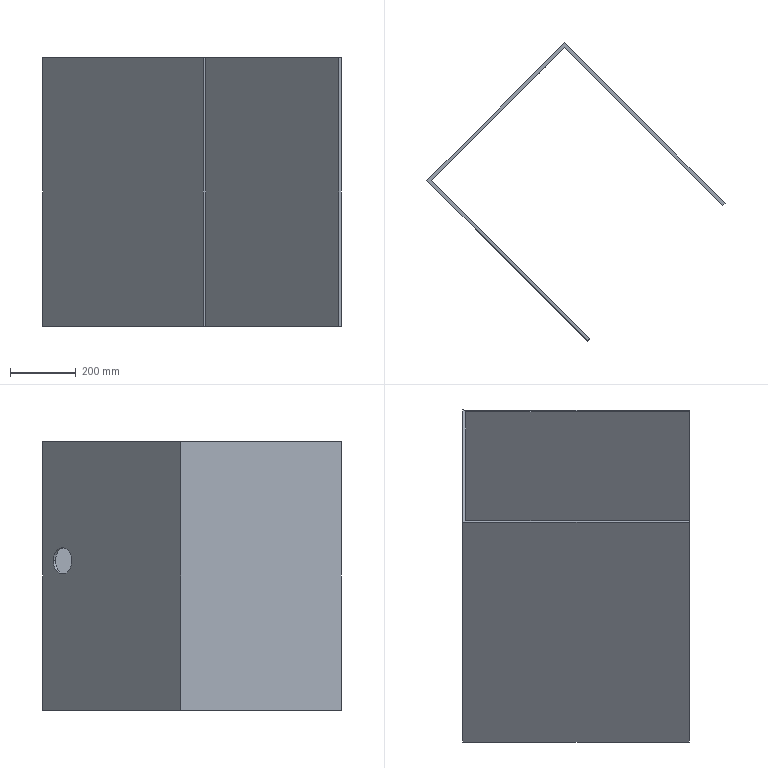Part | SolidWorks | 1 solid | 12 faces | box 906.604 x 906.604 x 817.42 mm | volume 15906852 mm3 | plane 10 | cylinder 2 | commonest cylinder face diameters 80 x2
STEP:
#1=CARTESIAN_POINT('',(76.071,429.624,-347.313));
#2=VERTEX_POINT('',#1);
#3=CARTESIAN_POINT('',(19.502,373.056,-347.313));
#4=VERTEX_POINT('',#3);
#5=CARTESIAN_POINT('',(47.787,401.34,-347.313));
#6=DIRECTION('',(-0.7071,0.7071,0.));
#7=DIRECTION('',(0.7071,0.7071,0.));
#8=AXIS2_PLACEMENT_3D('',#5,#6,#7);
#9=CIRCLE('',#8,40.);
#10=EDGE_CURVE('',#2,#4,#9,.T.);
#11=ORIENTED_EDGE('',*,*,#10,.T.);
#12=CARTESIAN_POINT('',(26.574,365.985,-347.313));
#13=VERTEX_POINT('',#12);
#14=CARTESIAN_POINT('',(19.502,373.056,-347.313));
#15=DIRECTION('',(0.7071,-0.7071,0.));
#16=VECTOR('',#15,1000.);
#17=LINE('',#14,#16);
#18=EDGE_CURVE('',#4,#13,#17,.T.);
#19=ORIENTED_EDGE('',*,*,#18,.T.);
#20=CARTESIAN_POINT('',(83.142,422.553,-347.313));
#21=VERTEX_POINT('',#20);
#22=CARTESIAN_POINT('',(54.858,394.269,-347.313));
#23=DIRECTION('',(0.7071,-0.7071,0.));
#24=DIRECTION('',(-0.7071,-0.7071,0.));
#25=AXIS2_PLACEMENT_3D('',#22,#23,#24);
#26=CIRCLE('',#25,40.);
#27=EDGE_CURVE('',#13,#21,#26,.T.);
#28=ORIENTED_EDGE('',*,*,#27,.T.);
#29=CARTESIAN_POINT('',(76.071,429.624,-347.313));
#30=DIRECTION('',(0.7071,-0.7071,0.));
#31=VECTOR('',#30,1000.);
#32=LINE('',#29,#31);
#33=EDGE_CURVE('',#2,#21,#32,.T.);
#34=ORIENTED_EDGE('',*,*,#33,.F.);
#35=EDGE_LOOP('',(#11,#19,#28,#34));
#36=FACE_OUTER_BOUND('',#35,.T.);
#37=CARTESIAN_POINT('',(54.858,394.269,-347.313));
#38=DIRECTION('',(-0.7071,0.7071,0.));
#39=DIRECTION('',(0.7071,0.7071,0.));
#40=AXIS2_PLACEMENT_3D('',#37,#38,#39);
#41=CYLINDRICAL_SURFACE('',#40,40.);
#42=ADVANCED_FACE('',(#36),#41,.F.);
#43=CARTESIAN_POINT('',(47.787,401.34,-347.313));
#44=DIRECTION('',(-0.7071,0.7071,0.));
#45=DIRECTION('',(-0.7071,-0.7071,0.));
#46=AXIS2_PLACEMENT_3D('',#43,#44,#45);
#47=CIRCLE('',#46,40.);
#48=EDGE_CURVE('',#4,#2,#47,.T.);
#49=ORIENTED_EDGE('',*,*,#48,.T.);
#50=ORIENTED_EDGE('',*,*,#33,.T.);
#51=CARTESIAN_POINT('',(54.858,394.269,-347.313));
#52=DIRECTION('',(0.7071,-0.7071,0.));
#53=DIRECTION('',(0.7071,0.7071,0.));
#54=AXIS2_PLACEMENT_3D('',#51,#52,#53);
#55=CIRCLE('',#54,40.);
#56=EDGE_CURVE('',#21,#13,#55,.T.);
#57=ORIENTED_EDGE('',*,*,#56,.T.);
#58=ORIENTED_EDGE('',*,*,#18,.F.);
#59=EDGE_LOOP('',(#49,#50,#57,#58));
#60=FACE_OUTER_BOUND('',#59,.T.);
#61=CARTESIAN_POINT('',(54.858,394.269,-347.313));
#62=DIRECTION('',(-0.7071,0.7071,0.));
#63=DIRECTION('',(0.7071,0.7071,0.));
#64=AXIS2_PLACEMENT_3D('',#61,#62,#63);
#65=CYLINDRICAL_SURFACE('',#64,40.);
#66=ADVANCED_FACE('',(#60),#65,.F.);
#67=ORIENTED_EDGE('',*,*,#10,.F.);
#68=ORIENTED_EDGE('',*,*,#48,.F.);
#69=EDGE_LOOP('',(#67,#68));
#70=FACE_BOUND('',#69,.T.);
#71=CARTESIAN_POINT('',(107.574,461.127,-802.42));
#72=VERTEX_POINT('',#71);
#73=CARTESIAN_POINT('',(-311.127,42.426,-802.42));
#74=VERTEX_POINT('',#73);
#75=CARTESIAN_POINT('',(107.574,461.127,-802.42));
#76=DIRECTION('',(-0.7071,-0.7071,0.));
#77=VECTOR('',#76,1000.);
#78=LINE('',#75,#77);
#79=EDGE_CURVE('',#72,#74,#78,.T.);
#80=ORIENTED_EDGE('',*,*,#79,.T.);
#81=CARTESIAN_POINT('',(-311.127,42.426,15.));
#82=VERTEX_POINT('',#81);
#83=CARTESIAN_POINT('',(-311.127,42.426,-802.42));
#84=DIRECTION('',(0.,0.,1.));
#85=VECTOR('',#84,1000.);
#86=LINE('',#83,#85);
#87=EDGE_CURVE('',#74,#82,#86,.T.);
#88=ORIENTED_EDGE('',*,*,#87,.T.);
#89=CARTESIAN_POINT('',(107.574,461.127,15.));
#90=VERTEX_POINT('',#89);
#91=CARTESIAN_POINT('',(-311.127,42.426,15.));
#92=DIRECTION('',(0.7071,0.7071,0.));
#93=VECTOR('',#92,1000.);
#94=LINE('',#91,#93);
#95=EDGE_CURVE('',#82,#90,#94,.T.);
#96=ORIENTED_EDGE('',*,*,#95,.T.);
#97=CARTESIAN_POINT('',(107.574,461.127,-802.42));
#98=DIRECTION('',(0.,0.,1.));
#99=VECTOR('',#98,1000.);
#100=LINE('',#97,#99);
#101=EDGE_CURVE('',#72,#90,#100,.T.);
#102=ORIENTED_EDGE('',*,*,#101,.F.);
#103=EDGE_LOOP('',(#80,#88,#96,#102));
#104=FACE_OUTER_BOUND('',#103,.T.);
#105=CARTESIAN_POINT('',(100.503,454.056,15.));
#106=DIRECTION('',(-0.7071,0.7071,0.));
#107=DIRECTION('',(0.,0.,1.));
#108=AXIS2_PLACEMENT_3D('',#105,#106,#107);
#109=PLANE('',#108);
#110=ADVANCED_FACE('',(#70,#104),#109,.T.);
#111=CARTESIAN_POINT('',(176.777,-445.477,-802.42));
#112=VERTEX_POINT('',#111);
#113=CARTESIAN_POINT('',(-311.127,42.426,-802.42));
#114=DIRECTION('',(0.7071,-0.7071,0.));
#115=VECTOR('',#114,1000.);
#116=LINE('',#113,#115);
#117=EDGE_CURVE('',#74,#112,#116,.T.);
#118=ORIENTED_EDGE('',*,*,#117,.T.);
#119=CARTESIAN_POINT('',(176.777,-445.477,15.));
#120=VERTEX_POINT('',#119);
#121=CARTESIAN_POINT('',(176.777,-445.477,-802.42));
#122=DIRECTION('',(0.,0.,1.));
#123=VECTOR('',#122,1000.);
#124=LINE('',#121,#123);
#125=EDGE_CURVE('',#112,#120,#124,.T.);
#126=ORIENTED_EDGE('',*,*,#125,.T.);
#127=CARTESIAN_POINT('',(176.777,-445.477,15.));
#128=DIRECTION('',(-0.7071,0.7071,0.));
#129=VECTOR('',#128,1000.);
#130=LINE('',#127,#129);
#131=EDGE_CURVE('',#120,#82,#130,.T.);
#132=ORIENTED_EDGE('',*,*,#131,.T.);
#133=ORIENTED_EDGE('',*,*,#87,.F.);
#134=EDGE_LOOP('',(#118,#126,#132,#133));
#135=FACE_OUTER_BOUND('',#134,.T.);
#136=CARTESIAN_POINT('',(-304.056,35.355,15.));
#137=DIRECTION('',(-0.7071,-0.7071,0.));
#138=DIRECTION('',(-0.7071,0.7071,0.));
#139=AXIS2_PLACEMENT_3D('',#136,#137,#138);
#140=PLANE('',#139);
#141=ADVANCED_FACE('',(#135),#140,.T.);
#142=CARTESIAN_POINT('',(595.477,-26.777,15.));
#143=VERTEX_POINT('',#142);
#144=CARTESIAN_POINT('',(588.406,-33.848,15.));
#145=VERTEX_POINT('',#144);
#146=CARTESIAN_POINT('',(595.477,-26.777,15.));
#147=DIRECTION('',(-0.7071,-0.7071,0.));
#148=VECTOR('',#147,1000.);
#149=LINE('',#146,#148);
#150=EDGE_CURVE('',#143,#145,#149,.T.);
#151=ORIENTED_EDGE('',*,*,#150,.F.);
#152=CARTESIAN_POINT('',(107.574,461.127,15.));
#153=DIRECTION('',(0.7071,-0.7071,0.));
#154=VECTOR('',#153,1000.);
#155=LINE('',#152,#154);
#156=EDGE_CURVE('',#90,#143,#155,.T.);
#157=ORIENTED_EDGE('',*,*,#156,.F.);
#158=ORIENTED_EDGE('',*,*,#95,.F.);
#159=ORIENTED_EDGE('',*,*,#131,.F.);
#160=CARTESIAN_POINT('',(183.848,-438.406,15.));
#161=VERTEX_POINT('',#160);
#162=CARTESIAN_POINT('',(183.848,-438.406,15.));
#163=DIRECTION('',(-0.7071,-0.7071,0.));
#164=VECTOR('',#163,1000.);
#165=LINE('',#162,#164);
#166=EDGE_CURVE('',#161,#120,#165,.T.);
#167=ORIENTED_EDGE('',*,*,#166,.F.);
#168=CARTESIAN_POINT('',(-296.985,42.426,15.));
#169=VERTEX_POINT('',#168);
#170=CARTESIAN_POINT('',(-296.985,42.426,15.));
#171=DIRECTION('',(0.7071,-0.7071,0.));
#172=VECTOR('',#171,1000.);
#173=LINE('',#170,#172);
#174=EDGE_CURVE('',#169,#161,#173,.T.);
#175=ORIENTED_EDGE('',*,*,#174,.F.);
#176=CARTESIAN_POINT('',(107.574,446.985,15.));
#177=VERTEX_POINT('',#176);
#178=CARTESIAN_POINT('',(107.574,446.985,15.));
#179=DIRECTION('',(-0.7071,-0.7071,0.));
#180=VECTOR('',#179,1000.);
#181=LINE('',#178,#180);
#182=EDGE_CURVE('',#177,#169,#181,.T.);
#183=ORIENTED_EDGE('',*,*,#182,.F.);
#184=CARTESIAN_POINT('',(588.406,-33.848,15.));
#185=DIRECTION('',(-0.7071,0.7071,0.));
#186=VECTOR('',#185,1000.);
#187=LINE('',#184,#186);
#188=EDGE_CURVE('',#145,#177,#187,.T.);
#189=ORIENTED_EDGE('',*,*,#188,.F.);
#190=EDGE_LOOP('',(#151,#157,#158,#159,#167,#175,#183,#189));
#191=FACE_OUTER_BOUND('',#190,.T.);
#192=CARTESIAN_POINT('',(-61.872,-199.758,15.));
#193=DIRECTION('',(0.,0.,1.));
#194=DIRECTION('',(1.,0.,0.));
#195=AXIS2_PLACEMENT_3D('',#192,#193,#194);
#196=PLANE('',#195);
#197=ADVANCED_FACE('',(#191),#196,.T.);
#198=ORIENTED_EDGE('',*,*,#125,.F.);
#199=CARTESIAN_POINT('',(183.848,-438.406,-802.42));
#200=VERTEX_POINT('',#199);
#201=CARTESIAN_POINT('',(176.777,-445.477,-802.42));
#202=DIRECTION('',(0.7071,0.7071,0.));
#203=VECTOR('',#202,1000.);
#204=LINE('',#201,#203);
#205=EDGE_CURVE('',#112,#200,#204,.T.);
#206=ORIENTED_EDGE('',*,*,#205,.T.);
#207=CARTESIAN_POINT('',(183.848,-438.406,-802.42));
#208=DIRECTION('',(0.,0.,1.));
#209=VECTOR('',#208,1000.);
#210=LINE('',#207,#209);
#211=EDGE_CURVE('',#200,#161,#210,.T.);
#212=ORIENTED_EDGE('',*,*,#211,.T.);
#213=ORIENTED_EDGE('',*,*,#166,.T.);
#214=EDGE_LOOP('',(#198,#206,#212,#213));
#215=FACE_OUTER_BOUND('',#214,.T.);
#216=CARTESIAN_POINT('',(180.312,-441.942,-393.71));
#217=DIRECTION('',(0.7071,-0.7071,0.));
#218=DIRECTION('',(0.,0.,-1.));
#219=AXIS2_PLACEMENT_3D('',#216,#217,#218);
#220=PLANE('',#219);
#221=ADVANCED_FACE('',(#215),#220,.T.);
#222=CARTESIAN_POINT('',(-296.985,42.426,-802.42));
#223=VERTEX_POINT('',#222);
#224=CARTESIAN_POINT('',(183.848,-438.406,-802.42));
#225=DIRECTION('',(-0.7071,0.7071,0.));
#226=VECTOR('',#225,1000.);
#227=LINE('',#224,#226);
#228=EDGE_CURVE('',#200,#223,#227,.T.);
#229=ORIENTED_EDGE('',*,*,#228,.T.);
#230=CARTESIAN_POINT('',(-296.985,42.426,-802.42));
#231=DIRECTION('',(0.,0.,1.));
#232=VECTOR('',#231,1000.);
#233=LINE('',#230,#232);
#234=EDGE_CURVE('',#223,#169,#233,.T.);
#235=ORIENTED_EDGE('',*,*,#234,.T.);
#236=ORIENTED_EDGE('',*,*,#174,.T.);
#237=ORIENTED_EDGE('',*,*,#211,.F.);
#238=EDGE_LOOP('',(#229,#235,#236,#237));
#239=FACE_OUTER_BOUND('',#238,.T.);
#240=CARTESIAN_POINT('',(-296.985,42.426,15.));
#241=DIRECTION('',(-0.7071,-0.7071,0.));
#242=DIRECTION('',(-0.7071,0.7071,0.));
#243=AXIS2_PLACEMENT_3D('',#240,#241,#242);
#244=PLANE('',#243);
#245=ADVANCED_FACE('',(#239),#244,.F.);
#246=ORIENTED_EDGE('',*,*,#27,.F.);
#247=ORIENTED_EDGE('',*,*,#56,.F.);
#248=EDGE_LOOP('',(#246,#247));
#249=FACE_BOUND('',#248,.T.);
#250=CARTESIAN_POINT('',(107.574,446.985,-802.42));
#251=VERTEX_POINT('',#250);
#252=CARTESIAN_POINT('',(-296.985,42.426,-802.42));
#253=DIRECTION('',(0.7071,0.7071,0.));
#254=VECTOR('',#253,1000.);
#255=LINE('',#252,#254);
#256=EDGE_CURVE('',#223,#251,#255,.T.);
#257=ORIENTED_EDGE('',*,*,#256,.T.);
#258=CARTESIAN_POINT('',(107.574,446.985,-802.42));
#259=DIRECTION('',(0.,0.,1.));
#260=VECTOR('',#259,1000.);
#261=LINE('',#258,#260);
#262=EDGE_CURVE('',#251,#177,#261,.T.);
#263=ORIENTED_EDGE('',*,*,#262,.T.);
#264=ORIENTED_EDGE('',*,*,#182,.T.);
#265=ORIENTED_EDGE('',*,*,#234,.F.);
#266=EDGE_LOOP('',(#257,#263,#264,#265));
#267=FACE_OUTER_BOUND('',#266,.T.);
#268=CARTESIAN_POINT('',(107.574,446.985,15.));
#269=DIRECTION('',(-0.7071,0.7071,0.));
#270=DIRECTION('',(0.,0.,1.));
#271=AXIS2_PLACEMENT_3D('',#268,#269,#270);
#272=PLANE('',#271);
#273=ADVANCED_FACE('',(#249,#267),#272,.F.);
#274=CARTESIAN_POINT('',(588.406,-33.848,-802.42));
#275=VERTEX_POINT('',#274);
#276=CARTESIAN_POINT('',(107.574,446.985,-802.42));
#277=DIRECTION('',(0.7071,-0.7071,0.));
#278=VECTOR('',#277,1000.);
#279=LINE('',#276,#278);
#280=EDGE_CURVE('',#251,#275,#279,.T.);
#281=ORIENTED_EDGE('',*,*,#280,.T.);
#282=CARTESIAN_POINT('',(588.406,-33.848,-802.42));
#283=DIRECTION('',(0.,0.,1.));
#284=VECTOR('',#283,1000.);
#285=LINE('',#282,#284);
#286=EDGE_CURVE('',#275,#145,#285,.T.);
#287=ORIENTED_EDGE('',*,*,#286,.T.);
#288=ORIENTED_EDGE('',*,*,#188,.T.);
#289=ORIENTED_EDGE('',*,*,#262,.F.);
#290=EDGE_LOOP('',(#281,#287,#288,#289));
#291=FACE_OUTER_BOUND('',#290,.T.);
#292=CARTESIAN_POINT('',(588.406,-33.848,15.));
#293=DIRECTION('',(0.7071,0.7071,0.));
#294=DIRECTION('',(0.,0.,-1.));
#295=AXIS2_PLACEMENT_3D('',#292,#293,#294);
#296=PLANE('',#295);
#297=ADVANCED_FACE('',(#291),#296,.F.);
#298=CARTESIAN_POINT('',(595.477,-26.777,-802.42));
#299=VERTEX_POINT('',#298);
#300=CARTESIAN_POINT('',(595.477,-26.777,-802.42));
#301=DIRECTION('',(0.,0.,1.));
#302=VECTOR('',#301,1000.);
#303=LINE('',#300,#302);
#304=EDGE_CURVE('',#299,#143,#303,.T.);
#305=ORIENTED_EDGE('',*,*,#304,.T.);
#306=ORIENTED_EDGE('',*,*,#150,.T.);
#307=ORIENTED_EDGE('',*,*,#286,.F.);
#308=CARTESIAN_POINT('',(588.406,-33.848,-802.42));
#309=DIRECTION('',(0.7071,0.7071,0.));
#310=VECTOR('',#309,1000.);
#311=LINE('',#308,#310);
#312=EDGE_CURVE('',#275,#299,#311,.T.);
#313=ORIENTED_EDGE('',*,*,#312,.T.);
#314=EDGE_LOOP('',(#305,#306,#307,#313));
#315=FACE_OUTER_BOUND('',#314,.T.);
#316=CARTESIAN_POINT('',(591.942,-30.312,-393.71));
#317=DIRECTION('',(-0.7071,0.7071,0.));
#318=DIRECTION('',(0.,0.,1.));
#319=AXIS2_PLACEMENT_3D('',#316,#317,#318);
#320=PLANE('',#319);
#321=ADVANCED_FACE('',(#315),#320,.F.);
#322=CARTESIAN_POINT('',(595.477,-26.777,-802.42));
#323=DIRECTION('',(-0.7071,0.7071,0.));
#324=VECTOR('',#323,1000.);
#325=LINE('',#322,#324);
#326=EDGE_CURVE('',#299,#72,#325,.T.);
#327=ORIENTED_EDGE('',*,*,#326,.T.);
#328=ORIENTED_EDGE('',*,*,#101,.T.);
#329=ORIENTED_EDGE('',*,*,#156,.T.);
#330=ORIENTED_EDGE('',*,*,#304,.F.);
#331=EDGE_LOOP('',(#327,#328,#329,#330));
#332=FACE_OUTER_BOUND('',#331,.T.);
#333=CARTESIAN_POINT('',(595.477,-26.777,15.));
#334=DIRECTION('',(0.7071,0.7071,0.));
#335=DIRECTION('',(0.,0.,-1.));
#336=AXIS2_PLACEMENT_3D('',#333,#334,#335);
#337=PLANE('',#336);
#338=ADVANCED_FACE('',(#332),#337,.T.);
#339=ORIENTED_EDGE('',*,*,#312,.F.);
#340=ORIENTED_EDGE('',*,*,#280,.F.);
#341=ORIENTED_EDGE('',*,*,#256,.F.);
#342=ORIENTED_EDGE('',*,*,#228,.F.);
#343=ORIENTED_EDGE('',*,*,#205,.F.);
#344=ORIENTED_EDGE('',*,*,#117,.F.);
#345=ORIENTED_EDGE('',*,*,#79,.F.);
#346=ORIENTED_EDGE('',*,*,#326,.F.);
#347=EDGE_LOOP('',(#339,#340,#341,#342,#343,#344,#345,#346));
#348=FACE_OUTER_BOUND('',#347,.T.);
#349=CARTESIAN_POINT('',(-61.872,-199.758,-802.42));
#350=DIRECTION('',(0.,0.,1.));
#351=DIRECTION('',(1.,0.,0.));
#352=AXIS2_PLACEMENT_3D('',#349,#350,#351);
#353=PLANE('',#352);
#354=ADVANCED_FACE('',(#348),#353,.F.);
#355=CLOSED_SHELL('',(#42,#66,#110,#141,#197,#221,#245,#273,#297,#321,#338,#354));
#356=MANIFOLD_SOLID_BREP('',#355);
#357=CARTESIAN_POINT('',(0.,0.,0.));
#358=DIRECTION('',(0.,0.,1.));
#359=DIRECTION('',(1.,0.,0.));
#360=AXIS2_PLACEMENT_3D('',#357,#358,#359);
#361=(LENGTH_UNIT()NAMED_UNIT(*)SI_UNIT(.MILLI.,.METRE.));
#362=UNCERTAINTY_MEASURE_WITH_UNIT(LENGTH_MEASURE(0.00001),#361,'','');
#363=(NAMED_UNIT(*)PLANE_ANGLE_UNIT()SI_UNIT($,.RADIAN.));
#364=(NAMED_UNIT(*)SI_UNIT($,.STERADIAN.)SOLID_ANGLE_UNIT());
#365=(GEOMETRIC_REPRESENTATION_CONTEXT(3)GLOBAL_UNCERTAINTY_ASSIGNED_CONTEXT((#362))GLOBAL_UNIT_ASSIGNED_CONTEXT((#361,#363,#364))REPRESENTATION_CONTEXT('',''));
#366=ADVANCED_BREP_SHAPE_REPRESENTATION('',(#356,#360),#365);